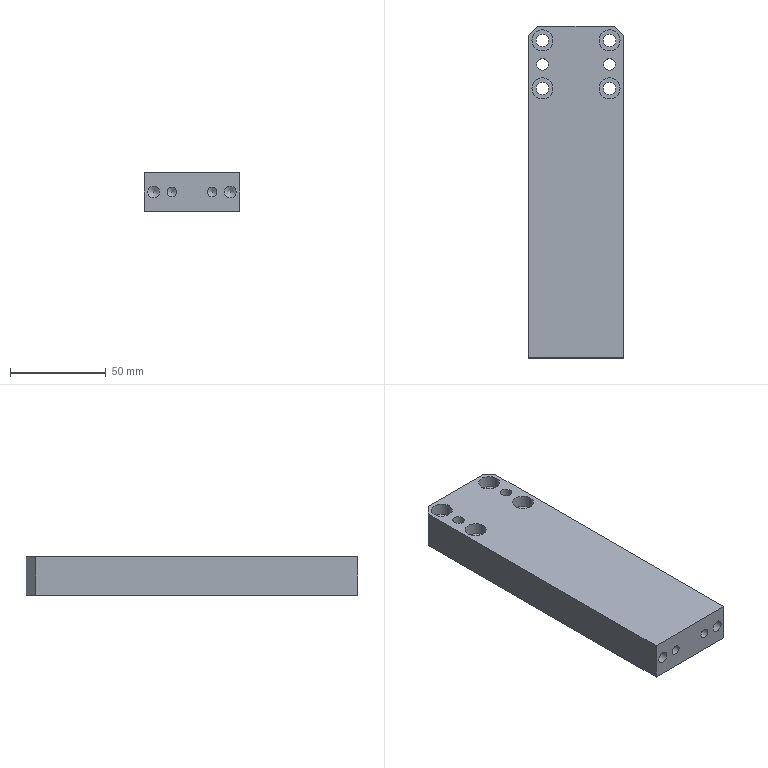Part | NX | features BREP 1 | 1 solid | 30 faces | box 50 x 173 x 20 mm | volume 165754 mm3 | cylinder 14 | plane 12 | cone 4 | commonest cylinder face diameters 6 x4 6.6 x4 11 x4 5 x2
STEP:
#1=CARTESIAN_POINT('',(-20.,86.5,0.));
#2=VERTEX_POINT('',#1);
#3=CARTESIAN_POINT('',(-25.,81.5,0.));
#4=VERTEX_POINT('',#3);
#5=CARTESIAN_POINT('',(-20.,86.5,0.));
#6=DIRECTION('',(-0.7071,-0.7071,0.));
#7=VECTOR('',#6,1000.);
#8=LINE('',#5,#7);
#9=EDGE_CURVE('',#2,#4,#8,.T.);
#10=ORIENTED_EDGE('',*,*,#9,.F.);
#11=CARTESIAN_POINT('',(20.,86.5,0.));
#12=VERTEX_POINT('',#11);
#13=CARTESIAN_POINT('',(0.,86.5,0.));
#14=DIRECTION('',(-1.,0.,0.));
#15=VECTOR('',#14,1000.);
#16=LINE('',#13,#15);
#17=EDGE_CURVE('',#12,#2,#16,.T.);
#18=ORIENTED_EDGE('',*,*,#17,.F.);
#19=CARTESIAN_POINT('',(25.,81.5,0.));
#20=VERTEX_POINT('',#19);
#21=CARTESIAN_POINT('',(25.,81.5,0.));
#22=DIRECTION('',(-0.7071,0.7071,0.));
#23=VECTOR('',#22,1000.);
#24=LINE('',#21,#23);
#25=EDGE_CURVE('',#20,#12,#24,.T.);
#26=ORIENTED_EDGE('',*,*,#25,.F.);
#27=CARTESIAN_POINT('',(25.,-86.5,0.));
#28=VERTEX_POINT('',#27);
#29=CARTESIAN_POINT('',(25.,0.,0.));
#30=DIRECTION('',(0.,1.,0.));
#31=VECTOR('',#30,1000.);
#32=LINE('',#29,#31);
#33=EDGE_CURVE('',#28,#20,#32,.T.);
#34=ORIENTED_EDGE('',*,*,#33,.F.);
#35=CARTESIAN_POINT('',(-25.,-86.5,0.));
#36=VERTEX_POINT('',#35);
#37=CARTESIAN_POINT('',(0.,-86.5,0.));
#38=DIRECTION('',(1.,0.,0.));
#39=VECTOR('',#38,1000.);
#40=LINE('',#37,#39);
#41=EDGE_CURVE('',#36,#28,#40,.T.);
#42=ORIENTED_EDGE('',*,*,#41,.F.);
#43=CARTESIAN_POINT('',(-25.,0.,0.));
#44=DIRECTION('',(0.,-1.,0.));
#45=VECTOR('',#44,1000.);
#46=LINE('',#43,#45);
#47=EDGE_CURVE('',#4,#36,#46,.T.);
#48=ORIENTED_EDGE('',*,*,#47,.F.);
#49=EDGE_LOOP('',(#10,#18,#26,#34,#42,#48));
#50=FACE_BOUND('',#49,.T.);
#51=CARTESIAN_POINT('',(-20.5,66.5,0.));
#52=VERTEX_POINT('',#51);
#53=CARTESIAN_POINT('',(-17.5,66.5,0.));
#54=DIRECTION('',(0.,0.,-1.));
#55=DIRECTION('',(-1.,0.,0.));
#56=AXIS2_PLACEMENT_3D('',#53,#54,#55);
#57=CIRCLE('',#56,3.);
#58=EDGE_CURVE('',#52,#52,#57,.T.);
#59=ORIENTED_EDGE('',*,*,#58,.F.);
#60=EDGE_LOOP('',(#59));
#61=FACE_BOUND('',#60,.T.);
#62=CARTESIAN_POINT('',(14.5,66.5,0.));
#63=VERTEX_POINT('',#62);
#64=CARTESIAN_POINT('',(17.5,66.5,0.));
#65=DIRECTION('',(0.,0.,-1.));
#66=DIRECTION('',(-1.,0.,0.));
#67=AXIS2_PLACEMENT_3D('',#64,#65,#66);
#68=CIRCLE('',#67,3.);
#69=EDGE_CURVE('',#63,#63,#68,.T.);
#70=ORIENTED_EDGE('',*,*,#69,.F.);
#71=EDGE_LOOP('',(#70));
#72=FACE_BOUND('',#71,.T.);
#73=CARTESIAN_POINT('',(-14.2,54.,0.));
#74=VERTEX_POINT('',#73);
#75=CARTESIAN_POINT('',(-17.5,54.,0.));
#76=DIRECTION('',(0.,0.,-1.));
#77=DIRECTION('',(1.,0.,0.));
#78=AXIS2_PLACEMENT_3D('',#75,#76,#77);
#79=CIRCLE('',#78,3.3);
#80=EDGE_CURVE('',#74,#74,#79,.T.);
#81=ORIENTED_EDGE('',*,*,#80,.F.);
#82=EDGE_LOOP('',(#81));
#83=FACE_BOUND('',#82,.T.);
#84=CARTESIAN_POINT('',(-14.2,79.,0.));
#85=VERTEX_POINT('',#84);
#86=CARTESIAN_POINT('',(-17.5,79.,0.));
#87=DIRECTION('',(0.,0.,-1.));
#88=DIRECTION('',(1.,0.,0.));
#89=AXIS2_PLACEMENT_3D('',#86,#87,#88);
#90=CIRCLE('',#89,3.3);
#91=EDGE_CURVE('',#85,#85,#90,.T.);
#92=ORIENTED_EDGE('',*,*,#91,.F.);
#93=EDGE_LOOP('',(#92));
#94=FACE_BOUND('',#93,.T.);
#95=CARTESIAN_POINT('',(20.8,54.,0.));
#96=VERTEX_POINT('',#95);
#97=CARTESIAN_POINT('',(17.5,54.,0.));
#98=DIRECTION('',(0.,0.,-1.));
#99=DIRECTION('',(1.,0.,0.));
#100=AXIS2_PLACEMENT_3D('',#97,#98,#99);
#101=CIRCLE('',#100,3.3);
#102=EDGE_CURVE('',#96,#96,#101,.T.);
#103=ORIENTED_EDGE('',*,*,#102,.F.);
#104=EDGE_LOOP('',(#103));
#105=FACE_BOUND('',#104,.T.);
#106=CARTESIAN_POINT('',(20.8,79.,0.));
#107=VERTEX_POINT('',#106);
#108=CARTESIAN_POINT('',(17.5,79.,0.));
#109=DIRECTION('',(0.,0.,-1.));
#110=DIRECTION('',(1.,0.,0.));
#111=AXIS2_PLACEMENT_3D('',#108,#109,#110);
#112=CIRCLE('',#111,3.3);
#113=EDGE_CURVE('',#107,#107,#112,.T.);
#114=ORIENTED_EDGE('',*,*,#113,.F.);
#115=EDGE_LOOP('',(#114));
#116=FACE_BOUND('',#115,.T.);
#117=CARTESIAN_POINT('',(0.,0.,0.));
#118=DIRECTION('',(0.,0.,1.));
#119=DIRECTION('',(-1.,0.,0.));
#120=AXIS2_PLACEMENT_3D('',#117,#118,#119);
#121=PLANE('',#120);
#122=ADVANCED_FACE('',(#50,#61,#72,#83,#94,#105,#116),#121,.F.);
#123=CARTESIAN_POINT('',(-25.,81.5,20.));
#124=VERTEX_POINT('',#123);
#125=CARTESIAN_POINT('',(-25.,81.5,20.));
#126=DIRECTION('',(0.,0.,1.));
#127=VECTOR('',#126,1000.);
#128=LINE('',#125,#127);
#129=EDGE_CURVE('',#4,#124,#128,.T.);
#130=ORIENTED_EDGE('',*,*,#129,.F.);
#131=ORIENTED_EDGE('',*,*,#47,.T.);
#132=CARTESIAN_POINT('',(-25.,-86.5,20.));
#133=VERTEX_POINT('',#132);
#134=CARTESIAN_POINT('',(-25.,-86.5,20.));
#135=DIRECTION('',(0.,0.,-1.));
#136=VECTOR('',#135,1000.);
#137=LINE('',#134,#136);
#138=EDGE_CURVE('',#133,#36,#137,.T.);
#139=ORIENTED_EDGE('',*,*,#138,.F.);
#140=CARTESIAN_POINT('',(-25.,86.5,20.));
#141=DIRECTION('',(0.,-1.,0.));
#142=VECTOR('',#141,1000.);
#143=LINE('',#140,#142);
#144=EDGE_CURVE('',#124,#133,#143,.T.);
#145=ORIENTED_EDGE('',*,*,#144,.F.);
#146=EDGE_LOOP('',(#130,#131,#139,#145));
#147=FACE_BOUND('',#146,.T.);
#148=CARTESIAN_POINT('',(-25.,86.5,20.));
#149=DIRECTION('',(1.,0.,0.));
#150=DIRECTION('',(0.,-1.,0.));
#151=AXIS2_PLACEMENT_3D('',#148,#149,#150);
#152=PLANE('',#151);
#153=ADVANCED_FACE('',(#147),#152,.F.);
#154=CARTESIAN_POINT('',(-20.,86.5,20.));
#155=VERTEX_POINT('',#154);
#156=CARTESIAN_POINT('',(-20.,86.5,20.));
#157=DIRECTION('',(0.,0.,1.));
#158=VECTOR('',#157,1000.);
#159=LINE('',#156,#158);
#160=EDGE_CURVE('',#2,#155,#159,.T.);
#161=ORIENTED_EDGE('',*,*,#160,.F.);
#162=ORIENTED_EDGE('',*,*,#9,.T.);
#163=ORIENTED_EDGE('',*,*,#129,.T.);
#164=CARTESIAN_POINT('',(-25.,81.5,20.));
#165=DIRECTION('',(-0.7071,-0.7071,0.));
#166=VECTOR('',#165,1000.);
#167=LINE('',#164,#166);
#168=EDGE_CURVE('',#155,#124,#167,.T.);
#169=ORIENTED_EDGE('',*,*,#168,.F.);
#170=EDGE_LOOP('',(#161,#162,#163,#169));
#171=FACE_BOUND('',#170,.T.);
#172=CARTESIAN_POINT('',(-25.,81.5,20.));
#173=DIRECTION('',(0.7071,-0.7071,0.));
#174=DIRECTION('',(-0.7071,-0.7071,0.));
#175=AXIS2_PLACEMENT_3D('',#172,#173,#174);
#176=PLANE('',#175);
#177=ADVANCED_FACE('',(#171),#176,.F.);
#178=ORIENTED_EDGE('',*,*,#160,.T.);
#179=CARTESIAN_POINT('',(20.,86.5,20.));
#180=VERTEX_POINT('',#179);
#181=CARTESIAN_POINT('',(-25.,86.5,20.));
#182=DIRECTION('',(-1.,0.,0.));
#183=VECTOR('',#182,1000.);
#184=LINE('',#181,#183);
#185=EDGE_CURVE('',#180,#155,#184,.T.);
#186=ORIENTED_EDGE('',*,*,#185,.F.);
#187=CARTESIAN_POINT('',(20.,86.5,20.));
#188=DIRECTION('',(0.,0.,1.));
#189=VECTOR('',#188,1000.);
#190=LINE('',#187,#189);
#191=EDGE_CURVE('',#12,#180,#190,.T.);
#192=ORIENTED_EDGE('',*,*,#191,.F.);
#193=ORIENTED_EDGE('',*,*,#17,.T.);
#194=EDGE_LOOP('',(#178,#186,#192,#193));
#195=FACE_BOUND('',#194,.T.);
#196=CARTESIAN_POINT('',(-25.,86.5,20.));
#197=DIRECTION('',(0.,-1.,0.));
#198=DIRECTION('',(0.,0.,1.));
#199=AXIS2_PLACEMENT_3D('',#196,#197,#198);
#200=PLANE('',#199);
#201=ADVANCED_FACE('',(#195),#200,.F.);
#202=CARTESIAN_POINT('',(25.,81.5,20.));
#203=VERTEX_POINT('',#202);
#204=CARTESIAN_POINT('',(25.,81.5,20.));
#205=DIRECTION('',(0.,0.,1.));
#206=VECTOR('',#205,1000.);
#207=LINE('',#204,#206);
#208=EDGE_CURVE('',#20,#203,#207,.T.);
#209=ORIENTED_EDGE('',*,*,#208,.F.);
#210=ORIENTED_EDGE('',*,*,#25,.T.);
#211=ORIENTED_EDGE('',*,*,#191,.T.);
#212=CARTESIAN_POINT('',(20.,86.5,20.));
#213=DIRECTION('',(-0.7071,0.7071,0.));
#214=VECTOR('',#213,1000.);
#215=LINE('',#212,#214);
#216=EDGE_CURVE('',#203,#180,#215,.T.);
#217=ORIENTED_EDGE('',*,*,#216,.F.);
#218=EDGE_LOOP('',(#209,#210,#211,#217));
#219=FACE_BOUND('',#218,.T.);
#220=CARTESIAN_POINT('',(20.,86.5,20.));
#221=DIRECTION('',(-0.7071,-0.7071,0.));
#222=DIRECTION('',(-0.7071,0.7071,0.));
#223=AXIS2_PLACEMENT_3D('',#220,#221,#222);
#224=PLANE('',#223);
#225=ADVANCED_FACE('',(#219),#224,.F.);
#226=ORIENTED_EDGE('',*,*,#208,.T.);
#227=CARTESIAN_POINT('',(25.,-86.5,20.));
#228=VERTEX_POINT('',#227);
#229=CARTESIAN_POINT('',(25.,86.5,20.));
#230=DIRECTION('',(0.,1.,0.));
#231=VECTOR('',#230,1000.);
#232=LINE('',#229,#231);
#233=EDGE_CURVE('',#228,#203,#232,.T.);
#234=ORIENTED_EDGE('',*,*,#233,.F.);
#235=CARTESIAN_POINT('',(25.,-86.5,20.));
#236=DIRECTION('',(0.,0.,1.));
#237=VECTOR('',#236,1000.);
#238=LINE('',#235,#237);
#239=EDGE_CURVE('',#28,#228,#238,.T.);
#240=ORIENTED_EDGE('',*,*,#239,.F.);
#241=ORIENTED_EDGE('',*,*,#33,.T.);
#242=EDGE_LOOP('',(#226,#234,#240,#241));
#243=FACE_BOUND('',#242,.T.);
#244=CARTESIAN_POINT('',(25.,86.5,20.));
#245=DIRECTION('',(-1.,0.,0.));
#246=DIRECTION('',(0.,1.,0.));
#247=AXIS2_PLACEMENT_3D('',#244,#245,#246);
#248=PLANE('',#247);
#249=ADVANCED_FACE('',(#243),#248,.F.);
#250=ORIENTED_EDGE('',*,*,#239,.T.);
#251=CARTESIAN_POINT('',(-25.,-86.5,20.));
#252=DIRECTION('',(1.,0.,0.));
#253=VECTOR('',#252,1000.);
#254=LINE('',#251,#253);
#255=EDGE_CURVE('',#133,#228,#254,.T.);
#256=ORIENTED_EDGE('',*,*,#255,.F.);
#257=ORIENTED_EDGE('',*,*,#138,.T.);
#258=ORIENTED_EDGE('',*,*,#41,.T.);
#259=EDGE_LOOP('',(#250,#256,#257,#258));
#260=FACE_BOUND('',#259,.T.);
#261=CARTESIAN_POINT('',(20.,-86.5,7.));
#262=VERTEX_POINT('',#261);
#263=CARTESIAN_POINT('',(20.,-86.5,10.));
#264=DIRECTION('',(0.,-1.,0.));
#265=DIRECTION('',(0.,0.,-1.));
#266=AXIS2_PLACEMENT_3D('',#263,#264,#265);
#267=CIRCLE('',#266,3.);
#268=EDGE_CURVE('',#262,#262,#267,.T.);
#269=ORIENTED_EDGE('',*,*,#268,.F.);
#270=EDGE_LOOP('',(#269));
#271=FACE_BOUND('',#270,.T.);
#272=CARTESIAN_POINT('',(-20.,-86.5,7.));
#273=VERTEX_POINT('',#272);
#274=CARTESIAN_POINT('',(-20.,-86.5,10.));
#275=DIRECTION('',(0.,-1.,0.));
#276=DIRECTION('',(0.,0.,-1.));
#277=AXIS2_PLACEMENT_3D('',#274,#275,#276);
#278=CIRCLE('',#277,3.);
#279=EDGE_CURVE('',#273,#273,#278,.T.);
#280=ORIENTED_EDGE('',*,*,#279,.F.);
#281=EDGE_LOOP('',(#280));
#282=FACE_BOUND('',#281,.T.);
#283=CARTESIAN_POINT('',(10.5,-86.5,7.5));
#284=VERTEX_POINT('',#283);
#285=CARTESIAN_POINT('',(10.5,-86.5,10.));
#286=DIRECTION('',(0.,-1.,0.));
#287=DIRECTION('',(0.,0.,-1.));
#288=AXIS2_PLACEMENT_3D('',#285,#286,#287);
#289=CIRCLE('',#288,2.5);
#290=EDGE_CURVE('',#284,#284,#289,.T.);
#291=ORIENTED_EDGE('',*,*,#290,.F.);
#292=EDGE_LOOP('',(#291));
#293=FACE_BOUND('',#292,.T.);
#294=CARTESIAN_POINT('',(-10.5,-86.5,7.5));
#295=VERTEX_POINT('',#294);
#296=CARTESIAN_POINT('',(-10.5,-86.5,10.));
#297=DIRECTION('',(0.,-1.,0.));
#298=DIRECTION('',(0.,0.,-1.));
#299=AXIS2_PLACEMENT_3D('',#296,#297,#298);
#300=CIRCLE('',#299,2.5);
#301=EDGE_CURVE('',#295,#295,#300,.T.);
#302=ORIENTED_EDGE('',*,*,#301,.F.);
#303=EDGE_LOOP('',(#302));
#304=FACE_BOUND('',#303,.T.);
#305=CARTESIAN_POINT('',(-25.,-86.5,20.));
#306=DIRECTION('',(0.,1.,0.));
#307=DIRECTION('',(0.,0.,-1.));
#308=AXIS2_PLACEMENT_3D('',#305,#306,#307);
#309=PLANE('',#308);
#310=ADVANCED_FACE('',(#260,#271,#282,#293,#304),#309,.F.);
#311=CARTESIAN_POINT('',(-20.5,66.5,20.));
#312=VERTEX_POINT('',#311);
#313=CARTESIAN_POINT('',(-17.5,66.5,20.));
#314=DIRECTION('',(0.,0.,-1.));
#315=DIRECTION('',(-1.,0.,0.));
#316=AXIS2_PLACEMENT_3D('',#313,#314,#315);
#317=CIRCLE('',#316,3.);
#318=EDGE_CURVE('',#312,#312,#317,.T.);
#319=ORIENTED_EDGE('',*,*,#318,.F.);
#320=EDGE_LOOP('',(#319));
#321=FACE_BOUND('',#320,.T.);
#322=ORIENTED_EDGE('',*,*,#58,.T.);
#323=EDGE_LOOP('',(#322));
#324=FACE_BOUND('',#323,.T.);
#325=CARTESIAN_POINT('',(-17.5,66.5,0.));
#326=DIRECTION('',(0.,0.,-1.));
#327=DIRECTION('',(1.,0.,0.));
#328=AXIS2_PLACEMENT_3D('',#325,#326,#327);
#329=CYLINDRICAL_SURFACE('',#328,3.);
#330=ADVANCED_FACE('',(#321,#324),#329,.F.);
#331=CARTESIAN_POINT('',(14.5,66.5,20.));
#332=VERTEX_POINT('',#331);
#333=CARTESIAN_POINT('',(17.5,66.5,20.));
#334=DIRECTION('',(0.,0.,-1.));
#335=DIRECTION('',(-1.,0.,0.));
#336=AXIS2_PLACEMENT_3D('',#333,#334,#335);
#337=CIRCLE('',#336,3.);
#338=EDGE_CURVE('',#332,#332,#337,.T.);
#339=ORIENTED_EDGE('',*,*,#338,.F.);
#340=EDGE_LOOP('',(#339));
#341=FACE_BOUND('',#340,.T.);
#342=ORIENTED_EDGE('',*,*,#69,.T.);
#343=EDGE_LOOP('',(#342));
#344=FACE_BOUND('',#343,.T.);
#345=CARTESIAN_POINT('',(17.5,66.5,0.));
#346=DIRECTION('',(0.,0.,-1.));
#347=DIRECTION('',(1.,0.,0.));
#348=AXIS2_PLACEMENT_3D('',#345,#346,#347);
#349=CYLINDRICAL_SURFACE('',#348,3.);
#350=ADVANCED_FACE('',(#341,#344),#349,.F.);
#351=ORIENTED_EDGE('',*,*,#80,.T.);
#352=EDGE_LOOP('',(#351));
#353=FACE_BOUND('',#352,.T.);
#354=CARTESIAN_POINT('',(-14.2,54.,13.6));
#355=VERTEX_POINT('',#354);
#356=CARTESIAN_POINT('',(-17.5,54.,13.6));
#357=DIRECTION('',(0.,0.,-1.));
#358=DIRECTION('',(1.,0.,0.));
#359=AXIS2_PLACEMENT_3D('',#356,#357,#358);
#360=CIRCLE('',#359,3.3);
#361=EDGE_CURVE('',#355,#355,#360,.T.);
#362=ORIENTED_EDGE('',*,*,#361,.F.);
#363=EDGE_LOOP('',(#362));
#364=FACE_BOUND('',#363,.T.);
#365=CARTESIAN_POINT('',(-17.5,54.,20.));
#366=DIRECTION('',(0.,0.,1.));
#367=DIRECTION('',(-1.,0.,0.));
#368=AXIS2_PLACEMENT_3D('',#365,#366,#367);
#369=CYLINDRICAL_SURFACE('',#368,3.3);
#370=ADVANCED_FACE('',(#353,#364),#369,.F.);
#371=ORIENTED_EDGE('',*,*,#91,.T.);
#372=EDGE_LOOP('',(#371));
#373=FACE_BOUND('',#372,.T.);
#374=CARTESIAN_POINT('',(-14.2,79.,13.6));
#375=VERTEX_POINT('',#374);
#376=CARTESIAN_POINT('',(-17.5,79.,13.6));
#377=DIRECTION('',(0.,0.,-1.));
#378=DIRECTION('',(1.,0.,0.));
#379=AXIS2_PLACEMENT_3D('',#376,#377,#378);
#380=CIRCLE('',#379,3.3);
#381=EDGE_CURVE('',#375,#375,#380,.T.);
#382=ORIENTED_EDGE('',*,*,#381,.F.);
#383=EDGE_LOOP('',(#382));
#384=FACE_BOUND('',#383,.T.);
#385=CARTESIAN_POINT('',(-17.5,79.,20.));
#386=DIRECTION('',(0.,0.,1.));
#387=DIRECTION('',(-1.,0.,0.));
#388=AXIS2_PLACEMENT_3D('',#385,#386,#387);
#389=CYLINDRICAL_SURFACE('',#388,3.3);
#390=ADVANCED_FACE('',(#373,#384),#389,.F.);
#391=ORIENTED_EDGE('',*,*,#102,.T.);
#392=EDGE_LOOP('',(#391));
#393=FACE_BOUND('',#392,.T.);
#394=CARTESIAN_POINT('',(20.8,54.,13.6));
#395=VERTEX_POINT('',#394);
#396=CARTESIAN_POINT('',(17.5,54.,13.6));
#397=DIRECTION('',(0.,0.,-1.));
#398=DIRECTION('',(1.,0.,0.));
#399=AXIS2_PLACEMENT_3D('',#396,#397,#398);
#400=CIRCLE('',#399,3.3);
#401=EDGE_CURVE('',#395,#395,#400,.T.);
#402=ORIENTED_EDGE('',*,*,#401,.F.);
#403=EDGE_LOOP('',(#402));
#404=FACE_BOUND('',#403,.T.);
#405=CARTESIAN_POINT('',(17.5,54.,20.));
#406=DIRECTION('',(0.,0.,1.));
#407=DIRECTION('',(-1.,0.,0.));
#408=AXIS2_PLACEMENT_3D('',#405,#406,#407);
#409=CYLINDRICAL_SURFACE('',#408,3.3);
#410=ADVANCED_FACE('',(#393,#404),#409,.F.);
#411=ORIENTED_EDGE('',*,*,#113,.T.);
#412=EDGE_LOOP('',(#411));
#413=FACE_BOUND('',#412,.T.);
#414=CARTESIAN_POINT('',(20.8,79.,13.6));
#415=VERTEX_POINT('',#414);
#416=CARTESIAN_POINT('',(17.5,79.,13.6));
#417=DIRECTION('',(0.,0.,-1.));
#418=DIRECTION('',(1.,0.,0.));
#419=AXIS2_PLACEMENT_3D('',#416,#417,#418);
#420=CIRCLE('',#419,3.3);
#421=EDGE_CURVE('',#415,#415,#420,.T.);
#422=ORIENTED_EDGE('',*,*,#421,.F.);
#423=EDGE_LOOP('',(#422));
#424=FACE_BOUND('',#423,.T.);
#425=CARTESIAN_POINT('',(17.5,79.,20.));
#426=DIRECTION('',(0.,0.,1.));
#427=DIRECTION('',(-1.,0.,0.));
#428=AXIS2_PLACEMENT_3D('',#425,#426,#427);
#429=CYLINDRICAL_SURFACE('',#428,3.3);
#430=ADVANCED_FACE('',(#413,#424),#429,.F.);
#431=ORIENTED_EDGE('',*,*,#233,.T.);
#432=ORIENTED_EDGE('',*,*,#216,.T.);
#433=ORIENTED_EDGE('',*,*,#185,.T.);
#434=ORIENTED_EDGE('',*,*,#168,.T.);
#435=ORIENTED_EDGE('',*,*,#144,.T.);
#436=ORIENTED_EDGE('',*,*,#255,.T.);
#437=EDGE_LOOP('',(#431,#432,#433,#434,#435,#436));
#438=FACE_BOUND('',#437,.T.);
#439=ORIENTED_EDGE('',*,*,#318,.T.);
#440=EDGE_LOOP('',(#439));
#441=FACE_BOUND('',#440,.T.);
#442=ORIENTED_EDGE('',*,*,#338,.T.);
#443=EDGE_LOOP('',(#442));
#444=FACE_BOUND('',#443,.T.);
#445=CARTESIAN_POINT('',(-12.,54.,20.));
#446=VERTEX_POINT('',#445);
#447=CARTESIAN_POINT('',(-17.5,54.,20.));
#448=DIRECTION('',(0.,0.,-1.));
#449=DIRECTION('',(1.,0.,0.));
#450=AXIS2_PLACEMENT_3D('',#447,#448,#449);
#451=CIRCLE('',#450,5.5);
#452=EDGE_CURVE('',#446,#446,#451,.T.);
#453=ORIENTED_EDGE('',*,*,#452,.T.);
#454=EDGE_LOOP('',(#453));
#455=FACE_BOUND('',#454,.T.);
#456=CARTESIAN_POINT('',(-12.,79.,20.));
#457=VERTEX_POINT('',#456);
#458=CARTESIAN_POINT('',(-17.5,79.,20.));
#459=DIRECTION('',(0.,0.,-1.));
#460=DIRECTION('',(1.,0.,0.));
#461=AXIS2_PLACEMENT_3D('',#458,#459,#460);
#462=CIRCLE('',#461,5.5);
#463=EDGE_CURVE('',#457,#457,#462,.T.);
#464=ORIENTED_EDGE('',*,*,#463,.T.);
#465=EDGE_LOOP('',(#464));
#466=FACE_BOUND('',#465,.T.);
#467=CARTESIAN_POINT('',(23.,54.,20.));
#468=VERTEX_POINT('',#467);
#469=CARTESIAN_POINT('',(17.5,54.,20.));
#470=DIRECTION('',(0.,0.,-1.));
#471=DIRECTION('',(1.,0.,0.));
#472=AXIS2_PLACEMENT_3D('',#469,#470,#471);
#473=CIRCLE('',#472,5.5);
#474=EDGE_CURVE('',#468,#468,#473,.T.);
#475=ORIENTED_EDGE('',*,*,#474,.T.);
#476=EDGE_LOOP('',(#475));
#477=FACE_BOUND('',#476,.T.);
#478=CARTESIAN_POINT('',(23.,79.,20.));
#479=VERTEX_POINT('',#478);
#480=CARTESIAN_POINT('',(17.5,79.,20.));
#481=DIRECTION('',(0.,0.,-1.));
#482=DIRECTION('',(1.,0.,0.));
#483=AXIS2_PLACEMENT_3D('',#480,#481,#482);
#484=CIRCLE('',#483,5.5);
#485=EDGE_CURVE('',#479,#479,#484,.T.);
#486=ORIENTED_EDGE('',*,*,#485,.T.);
#487=EDGE_LOOP('',(#486));
#488=FACE_BOUND('',#487,.T.);
#489=CARTESIAN_POINT('',(0.,0.,20.));
#490=DIRECTION('',(0.,0.,1.));
#491=DIRECTION('',(-1.,0.,0.));
#492=AXIS2_PLACEMENT_3D('',#489,#490,#491);
#493=PLANE('',#492);
#494=ADVANCED_FACE('',(#438,#441,#444,#455,#466,#477,#488),#493,.T.);
#495=CARTESIAN_POINT('',(20.,-74.5,7.));
#496=VERTEX_POINT('',#495);
#497=CARTESIAN_POINT('',(20.,-74.5,10.));
#498=DIRECTION('',(0.,-1.,0.));
#499=DIRECTION('',(0.,0.,-1.));
#500=AXIS2_PLACEMENT_3D('',#497,#498,#499);
#501=CIRCLE('',#500,3.);
#502=EDGE_CURVE('',#496,#496,#501,.T.);
#503=ORIENTED_EDGE('',*,*,#502,.F.);
#504=EDGE_LOOP('',(#503));
#505=FACE_BOUND('',#504,.T.);
#506=ORIENTED_EDGE('',*,*,#268,.T.);
#507=EDGE_LOOP('',(#506));
#508=FACE_BOUND('',#507,.T.);
#509=CARTESIAN_POINT('',(20.,-86.5,10.));
#510=DIRECTION('',(0.,-1.,0.));
#511=DIRECTION('',(0.,0.,1.));
#512=AXIS2_PLACEMENT_3D('',#509,#510,#511);
#513=CYLINDRICAL_SURFACE('',#512,3.);
#514=ADVANCED_FACE('',(#505,#508),#513,.F.);
#515=CARTESIAN_POINT('',(-20.,-74.5,7.));
#516=VERTEX_POINT('',#515);
#517=CARTESIAN_POINT('',(-20.,-74.5,10.));
#518=DIRECTION('',(0.,-1.,0.));
#519=DIRECTION('',(0.,0.,-1.));
#520=AXIS2_PLACEMENT_3D('',#517,#518,#519);
#521=CIRCLE('',#520,3.);
#522=EDGE_CURVE('',#516,#516,#521,.T.);
#523=ORIENTED_EDGE('',*,*,#522,.F.);
#524=EDGE_LOOP('',(#523));
#525=FACE_BOUND('',#524,.T.);
#526=ORIENTED_EDGE('',*,*,#279,.T.);
#527=EDGE_LOOP('',(#526));
#528=FACE_BOUND('',#527,.T.);
#529=CARTESIAN_POINT('',(-20.,-86.5,10.));
#530=DIRECTION('',(0.,-1.,0.));
#531=DIRECTION('',(0.,0.,1.));
#532=AXIS2_PLACEMENT_3D('',#529,#530,#531);
#533=CYLINDRICAL_SURFACE('',#532,3.);
#534=ADVANCED_FACE('',(#525,#528),#533,.F.);
#535=CARTESIAN_POINT('',(10.5,-71.5,7.5));
#536=VERTEX_POINT('',#535);
#537=CARTESIAN_POINT('',(10.5,-71.5,10.));
#538=DIRECTION('',(0.,-1.,0.));
#539=DIRECTION('',(0.,0.,-1.));
#540=AXIS2_PLACEMENT_3D('',#537,#538,#539);
#541=CIRCLE('',#540,2.5);
#542=EDGE_CURVE('',#536,#536,#541,.T.);
#543=ORIENTED_EDGE('',*,*,#542,.F.);
#544=EDGE_LOOP('',(#543));
#545=FACE_BOUND('',#544,.T.);
#546=ORIENTED_EDGE('',*,*,#290,.T.);
#547=EDGE_LOOP('',(#546));
#548=FACE_BOUND('',#547,.T.);
#549=CARTESIAN_POINT('',(10.5,-86.5,10.));
#550=DIRECTION('',(0.,-1.,0.));
#551=DIRECTION('',(0.,0.,1.));
#552=AXIS2_PLACEMENT_3D('',#549,#550,#551);
#553=CYLINDRICAL_SURFACE('',#552,2.5);
#554=ADVANCED_FACE('',(#545,#548),#553,.F.);
#555=CARTESIAN_POINT('',(-10.5,-71.5,7.5));
#556=VERTEX_POINT('',#555);
#557=CARTESIAN_POINT('',(-10.5,-71.5,10.));
#558=DIRECTION('',(0.,-1.,0.));
#559=DIRECTION('',(0.,0.,-1.));
#560=AXIS2_PLACEMENT_3D('',#557,#558,#559);
#561=CIRCLE('',#560,2.5);
#562=EDGE_CURVE('',#556,#556,#561,.T.);
#563=ORIENTED_EDGE('',*,*,#562,.F.);
#564=EDGE_LOOP('',(#563));
#565=FACE_BOUND('',#564,.T.);
#566=ORIENTED_EDGE('',*,*,#301,.T.);
#567=EDGE_LOOP('',(#566));
#568=FACE_BOUND('',#567,.T.);
#569=CARTESIAN_POINT('',(-10.5,-86.5,10.));
#570=DIRECTION('',(0.,-1.,0.));
#571=DIRECTION('',(0.,0.,1.));
#572=AXIS2_PLACEMENT_3D('',#569,#570,#571);
#573=CYLINDRICAL_SURFACE('',#572,2.5);
#574=ADVANCED_FACE('',(#565,#568),#573,.F.);
#575=CARTESIAN_POINT('',(-12.,54.,13.6));
#576=VERTEX_POINT('',#575);
#577=CARTESIAN_POINT('',(-17.5,54.,13.6));
#578=DIRECTION('',(0.,0.,-1.));
#579=DIRECTION('',(1.,0.,0.));
#580=AXIS2_PLACEMENT_3D('',#577,#578,#579);
#581=CIRCLE('',#580,5.5);
#582=EDGE_CURVE('',#576,#576,#581,.T.);
#583=ORIENTED_EDGE('',*,*,#582,.F.);
#584=EDGE_LOOP('',(#583));
#585=FACE_BOUND('',#584,.T.);
#586=ORIENTED_EDGE('',*,*,#361,.T.);
#587=EDGE_LOOP('',(#586));
#588=FACE_BOUND('',#587,.T.);
#589=CARTESIAN_POINT('',(-14.2,54.,13.6));
#590=DIRECTION('',(0.,0.,-1.));
#591=DIRECTION('',(1.,0.,0.));
#592=AXIS2_PLACEMENT_3D('',#589,#590,#591);
#593=PLANE('',#592);
#594=ADVANCED_FACE('',(#585,#588),#593,.F.);
#595=CARTESIAN_POINT('',(-12.,79.,13.6));
#596=VERTEX_POINT('',#595);
#597=CARTESIAN_POINT('',(-17.5,79.,13.6));
#598=DIRECTION('',(0.,0.,-1.));
#599=DIRECTION('',(1.,0.,0.));
#600=AXIS2_PLACEMENT_3D('',#597,#598,#599);
#601=CIRCLE('',#600,5.5);
#602=EDGE_CURVE('',#596,#596,#601,.T.);
#603=ORIENTED_EDGE('',*,*,#602,.F.);
#604=EDGE_LOOP('',(#603));
#605=FACE_BOUND('',#604,.T.);
#606=ORIENTED_EDGE('',*,*,#381,.T.);
#607=EDGE_LOOP('',(#606));
#608=FACE_BOUND('',#607,.T.);
#609=CARTESIAN_POINT('',(-14.2,79.,13.6));
#610=DIRECTION('',(0.,0.,-1.));
#611=DIRECTION('',(1.,0.,0.));
#612=AXIS2_PLACEMENT_3D('',#609,#610,#611);
#613=PLANE('',#612);
#614=ADVANCED_FACE('',(#605,#608),#613,.F.);
#615=CARTESIAN_POINT('',(23.,54.,13.6));
#616=VERTEX_POINT('',#615);
#617=CARTESIAN_POINT('',(17.5,54.,13.6));
#618=DIRECTION('',(0.,0.,-1.));
#619=DIRECTION('',(1.,0.,0.));
#620=AXIS2_PLACEMENT_3D('',#617,#618,#619);
#621=CIRCLE('',#620,5.5);
#622=EDGE_CURVE('',#616,#616,#621,.T.);
#623=ORIENTED_EDGE('',*,*,#622,.F.);
#624=EDGE_LOOP('',(#623));
#625=FACE_BOUND('',#624,.T.);
#626=ORIENTED_EDGE('',*,*,#401,.T.);
#627=EDGE_LOOP('',(#626));
#628=FACE_BOUND('',#627,.T.);
#629=CARTESIAN_POINT('',(20.8,54.,13.6));
#630=DIRECTION('',(0.,0.,-1.));
#631=DIRECTION('',(1.,0.,0.));
#632=AXIS2_PLACEMENT_3D('',#629,#630,#631);
#633=PLANE('',#632);
#634=ADVANCED_FACE('',(#625,#628),#633,.F.);
#635=CARTESIAN_POINT('',(23.,79.,13.6));
#636=VERTEX_POINT('',#635);
#637=CARTESIAN_POINT('',(17.5,79.,13.6));
#638=DIRECTION('',(0.,0.,-1.));
#639=DIRECTION('',(1.,0.,0.));
#640=AXIS2_PLACEMENT_3D('',#637,#638,#639);
#641=CIRCLE('',#640,5.5);
#642=EDGE_CURVE('',#636,#636,#641,.T.);
#643=ORIENTED_EDGE('',*,*,#642,.F.);
#644=EDGE_LOOP('',(#643));
#645=FACE_BOUND('',#644,.T.);
#646=ORIENTED_EDGE('',*,*,#421,.T.);
#647=EDGE_LOOP('',(#646));
#648=FACE_BOUND('',#647,.T.);
#649=CARTESIAN_POINT('',(20.8,79.,13.6));
#650=DIRECTION('',(0.,0.,-1.));
#651=DIRECTION('',(1.,0.,0.));
#652=AXIS2_PLACEMENT_3D('',#649,#650,#651);
#653=PLANE('',#652);
#654=ADVANCED_FACE('',(#645,#648),#653,.F.);
#655=ORIENTED_EDGE('',*,*,#452,.F.);
#656=EDGE_LOOP('',(#655));
#657=FACE_BOUND('',#656,.T.);
#658=ORIENTED_EDGE('',*,*,#582,.T.);
#659=EDGE_LOOP('',(#658));
#660=FACE_BOUND('',#659,.T.);
#661=CARTESIAN_POINT('',(-17.5,54.,20.));
#662=DIRECTION('',(0.,0.,1.));
#663=DIRECTION('',(-1.,0.,0.));
#664=AXIS2_PLACEMENT_3D('',#661,#662,#663);
#665=CYLINDRICAL_SURFACE('',#664,5.5);
#666=ADVANCED_FACE('',(#657,#660),#665,.F.);
#667=ORIENTED_EDGE('',*,*,#463,.F.);
#668=EDGE_LOOP('',(#667));
#669=FACE_BOUND('',#668,.T.);
#670=ORIENTED_EDGE('',*,*,#602,.T.);
#671=EDGE_LOOP('',(#670));
#672=FACE_BOUND('',#671,.T.);
#673=CARTESIAN_POINT('',(-17.5,79.,20.));
#674=DIRECTION('',(0.,0.,1.));
#675=DIRECTION('',(-1.,0.,0.));
#676=AXIS2_PLACEMENT_3D('',#673,#674,#675);
#677=CYLINDRICAL_SURFACE('',#676,5.5);
#678=ADVANCED_FACE('',(#669,#672),#677,.F.);
#679=ORIENTED_EDGE('',*,*,#474,.F.);
#680=EDGE_LOOP('',(#679));
#681=FACE_BOUND('',#680,.T.);
#682=ORIENTED_EDGE('',*,*,#622,.T.);
#683=EDGE_LOOP('',(#682));
#684=FACE_BOUND('',#683,.T.);
#685=CARTESIAN_POINT('',(17.5,54.,20.));
#686=DIRECTION('',(0.,0.,1.));
#687=DIRECTION('',(-1.,0.,0.));
#688=AXIS2_PLACEMENT_3D('',#685,#686,#687);
#689=CYLINDRICAL_SURFACE('',#688,5.5);
#690=ADVANCED_FACE('',(#681,#684),#689,.F.);
#691=ORIENTED_EDGE('',*,*,#485,.F.);
#692=EDGE_LOOP('',(#691));
#693=FACE_BOUND('',#692,.T.);
#694=ORIENTED_EDGE('',*,*,#642,.T.);
#695=EDGE_LOOP('',(#694));
#696=FACE_BOUND('',#695,.T.);
#697=CARTESIAN_POINT('',(17.5,79.,20.));
#698=DIRECTION('',(0.,0.,1.));
#699=DIRECTION('',(-1.,0.,0.));
#700=AXIS2_PLACEMENT_3D('',#697,#698,#699);
#701=CYLINDRICAL_SURFACE('',#700,5.5);
#702=ADVANCED_FACE('',(#693,#696),#701,.F.);
#703=CARTESIAN_POINT('',(20.,-72.697,10.));
#704=VERTEX_POINT('',#703);
#705=VERTEX_LOOP('',#704);
#706=FACE_BOUND('',#705,.T.);
#707=ORIENTED_EDGE('',*,*,#502,.T.);
#708=EDGE_LOOP('',(#707));
#709=FACE_BOUND('',#708,.T.);
#710=CARTESIAN_POINT('',(20.,-74.5,10.));
#711=DIRECTION('',(0.,-1.,0.));
#712=DIRECTION('',(0.,0.,1.));
#713=AXIS2_PLACEMENT_3D('',#710,#711,#712);
#714=CONICAL_SURFACE('',#713,3.,1.03);
#715=ADVANCED_FACE('',(#706,#709),#714,.F.);
#716=CARTESIAN_POINT('',(-20.,-72.697,10.));
#717=VERTEX_POINT('',#716);
#718=VERTEX_LOOP('',#717);
#719=FACE_BOUND('',#718,.T.);
#720=ORIENTED_EDGE('',*,*,#522,.T.);
#721=EDGE_LOOP('',(#720));
#722=FACE_BOUND('',#721,.T.);
#723=CARTESIAN_POINT('',(-20.,-74.5,10.));
#724=DIRECTION('',(0.,-1.,0.));
#725=DIRECTION('',(0.,0.,1.));
#726=AXIS2_PLACEMENT_3D('',#723,#724,#725);
#727=CONICAL_SURFACE('',#726,3.,1.03);
#728=ADVANCED_FACE('',(#719,#722),#727,.F.);
#729=CARTESIAN_POINT('',(10.5,-69.998,10.));
#730=VERTEX_POINT('',#729);
#731=VERTEX_LOOP('',#730);
#732=FACE_BOUND('',#731,.T.);
#733=ORIENTED_EDGE('',*,*,#542,.T.);
#734=EDGE_LOOP('',(#733));
#735=FACE_BOUND('',#734,.T.);
#736=CARTESIAN_POINT('',(10.5,-71.5,10.));
#737=DIRECTION('',(0.,-1.,0.));
#738=DIRECTION('',(0.,0.,1.));
#739=AXIS2_PLACEMENT_3D('',#736,#737,#738);
#740=CONICAL_SURFACE('',#739,2.5,1.03);
#741=ADVANCED_FACE('',(#732,#735),#740,.F.);
#742=CARTESIAN_POINT('',(-10.5,-69.998,10.));
#743=VERTEX_POINT('',#742);
#744=VERTEX_LOOP('',#743);
#745=FACE_BOUND('',#744,.T.);
#746=ORIENTED_EDGE('',*,*,#562,.T.);
#747=EDGE_LOOP('',(#746));
#748=FACE_BOUND('',#747,.T.);
#749=CARTESIAN_POINT('',(-10.5,-71.5,10.));
#750=DIRECTION('',(0.,-1.,0.));
#751=DIRECTION('',(0.,0.,1.));
#752=AXIS2_PLACEMENT_3D('',#749,#750,#751);
#753=CONICAL_SURFACE('',#752,2.5,1.03);
#754=ADVANCED_FACE('',(#745,#748),#753,.F.);
#755=CLOSED_SHELL('',(#122,#153,#177,#201,#225,#249,#310,#330,#350,#370,#390,#410,#430,#494,#514,#534,#554,#574,#594,#614,#634,#654,#666,#678,#690,#702,#715,#728,#741,#754));
#756=MANIFOLD_SOLID_BREP('',#755);
#757=(LENGTH_UNIT()NAMED_UNIT(*)SI_UNIT(.MILLI.,.METRE.));
#758=UNCERTAINTY_MEASURE_WITH_UNIT(LENGTH_MEASURE(0.00001),#757,'','');
#759=(NAMED_UNIT(*)PLANE_ANGLE_UNIT()SI_UNIT($,.RADIAN.));
#760=(NAMED_UNIT(*)SI_UNIT($,.STERADIAN.)SOLID_ANGLE_UNIT());
#761=(GEOMETRIC_REPRESENTATION_CONTEXT(3)GLOBAL_UNCERTAINTY_ASSIGNED_CONTEXT((#758))GLOBAL_UNIT_ASSIGNED_CONTEXT((#757,#759,#760))REPRESENTATION_CONTEXT('',''));
#762=ADVANCED_BREP_SHAPE_REPRESENTATION('',(#756),#761);